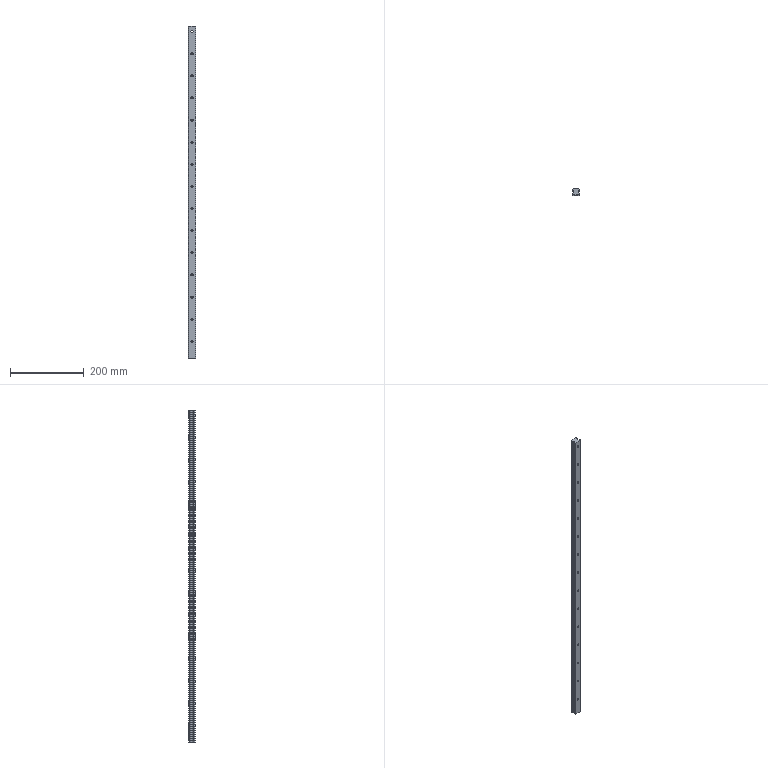Part | STEP file | Mirror HGR20_3_AF0 | 1 solid | 119 faces | box 20 x 17.5 x 900 mm | volume 257708 mm3 | cylinder 82 | plane 37 | commonest cylinder face diameters 5.5 x24 10 x24 1 x12 2 x6 6 x6 9.5 x6